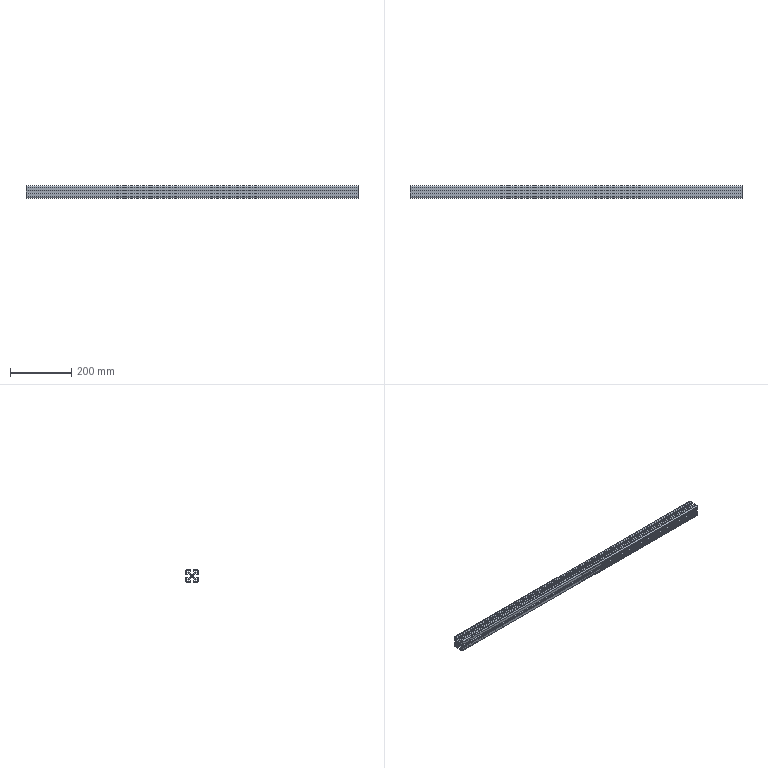Part | STEP file | Profile MK-8-4040C-L-00 4040C standard 1086mm | 1 solid | 188 faces | box 1086 x 40 x 40 mm | volume 519378 mm3 | cylinder 94 | plane 94 | commonest cylinder face diameters 0.6 x30 2 x28 4 x16 0.4 x8 6 x4 9 x4